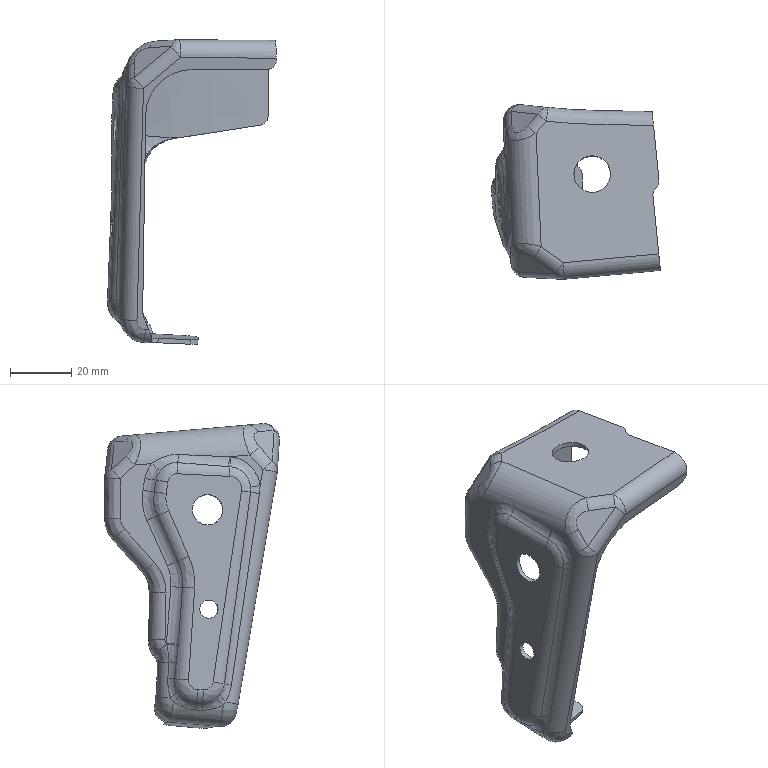Part | 1 solid | 222 faces | box 55.268 x 57.221 x 99.722 mm | volume 12742 mm3 | spline 135 | cylinder 56 | plane 23 | sphere 8 | commonest cylinder face diameters 10 x23 7 x20 20 x3 6 x2 12 x2 13 x2